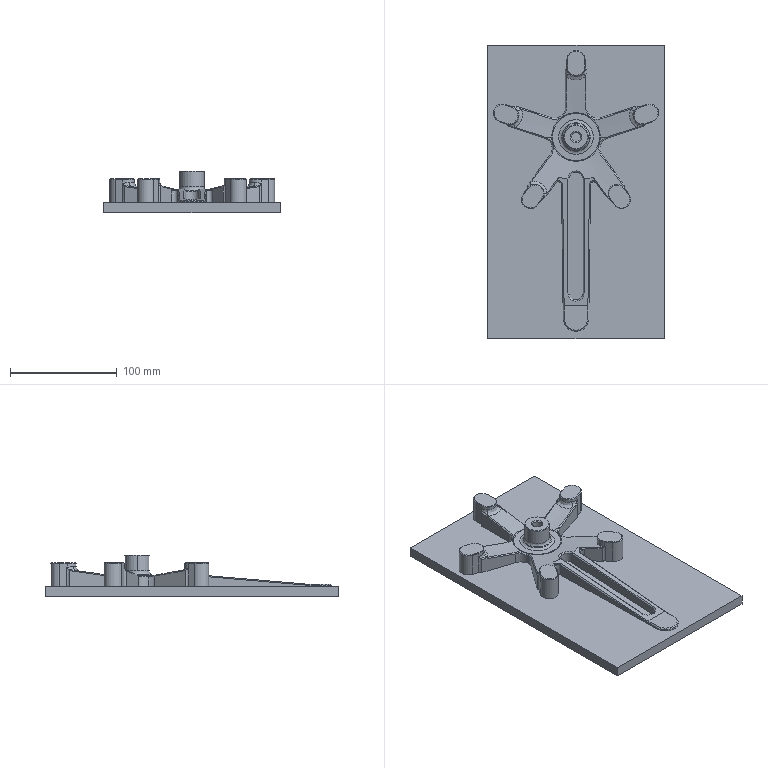NC program | NX | posted with a generic post | part box 165 x 275 x 39 mm
Lines 1 to 1483 of 70117:
N10 G17 G21 G94 G90
(CAVITY_MILL , TOOL : D12)
N12 T00 M6
N14 G54
N16 G17 G0 G90 X0. Y-200.696 S0 M3
N18 G43 Z30. H0
N20 Z2.523
N22 G94 G1 Z-0.477 F250.
N24 Y-189.296
N26 X-82.505
N28 X-82.595 Y-189.281
N30 G2 X-82.781 Y-189.096 R0.471
N32 G1 X-82.796 Y-189.006
N34 Y86.009
N36 G2 X-82.509 Y86.296 R0.293
N38 G1 X82.508
N40 G2 X82.796 Y86.009 R0.293
N42 G1 Y-189.009
N44 G2 X82.508 Y-189.296 R0.293
N46 G1 X0.
N48 Y-183.296
N50 X-76.796
N52 Y80.296
N54 X76.796
N56 Y-183.296
N58 X0.
N60 Y-177.296
N62 X-70.796
N64 Y74.296
N66 X70.796
N68 Y-177.296
N70 X0.
N72 Y-171.296
N74 X-64.796
N76 Y68.296
N78 X64.796
N80 Y-171.296
N82 X0.
N84 Y-165.296
N86 X-58.796
N88 Y62.296
N90 X58.796
N92 Y-165.296
N94 X0.
N96 Y-159.296
N98 X-52.796
N100 Y56.296
N102 X52.796
N104 Y-159.296
N106 X0.
N108 Y-153.296
N110 X-46.796
N112 Y50.296
N114 X46.796
N116 Y-153.296
N118 X0.
N120 Y-147.296
N122 X-40.796
N124 Y44.296
N126 X40.796
N128 Y-147.296
N130 X0.
N132 Y-141.296
N134 X-34.796
N136 Y38.296
N138 X34.796
N140 Y-141.296
N142 X0.
N144 Y-135.296
N146 X-28.796
N148 Y32.296
N150 X28.796
N152 Y-135.296
N154 X0.
N156 Y-129.296
N158 X-22.796
N160 Y26.296
N162 X22.796
N164 Y8.168
N166 X16.796
N168 G3 X-16.796 Y8.168 R18.677
N170 G1 Y20.296
N172 X16.796
N174 Y8.168
N176 X22.796
N178 Y-129.296
N180 X0.
N182 Y-123.296
N184 X-16.796
N186 Y-8.168
N188 G3 X16.796 Y-8.168 R18.677
N190 G1 X15.717 Y-7.643
N192 G2 X-7.643 Y-15.717 R17.477
N194 X15.717 Y-7.643 R-17.477
N196 G1 X16.796 Y-8.168
N198 Y-123.296
N200 X0.
N202 Y-117.296
N204 X-10.796
N206 Y-22.19
N208 G3 X10.796 Y-22.19 R24.677
N210 G1 Y-117.296
N212 X0.
N214 Y-111.296
N216 X-4.796
N218 Y-30.299
N220 G3 X4.796 Y-30.299 R30.677
N222 G1 Y-111.296
N224 X0.
N226 Y-117.296
N228 Z2.523
N230 G0 Z3.
N232 Y-200.696
N234 Z2.047
N236 G1 Z-0.953
N238 Y-189.296
N240 X-82.505
N242 X-82.595 Y-189.281
N244 G2 X-82.781 Y-189.096 R0.471
N246 G1 X-82.796 Y-189.006
N248 Y86.009
N250 G2 X-82.509 Y86.296 R0.293
N252 G1 X82.509
N254 G2 X82.796 Y86.009 R0.293
N256 G1 Y-189.009
N258 G2 X82.508 Y-189.296 R0.293
N260 G1 X0.
N262 Y-183.296
N264 X-76.796
N266 Y80.296
N268 X76.796
N270 Y-183.296
N272 X0.
N274 Y-177.296
N276 X-70.796
N278 Y74.296
N280 X70.796
N282 Y-177.296
N284 X0.
N286 Y-171.296
N288 X-64.796
N290 Y68.296
N292 X64.796
N294 Y-171.296
N296 X0.
N298 Y-165.296
N300 X-58.796
N302 Y62.296
N304 X58.796
N306 Y-165.296
N308 X0.
N310 Y-159.296
N312 X-52.796
N314 Y56.296
N316 X52.796
N318 Y-159.296
N320 X0.
N322 Y-153.296
N324 X-46.796
N326 Y50.296
N328 X46.796
N330 Y-153.296
N332 X0.
N334 Y-147.296
N336 X-40.796
N338 Y44.296
N340 X40.796
N342 Y-147.296
N344 X0.
N346 Y-141.296
N348 X-34.796
N350 Y38.296
N352 X34.796
N354 Y-141.296
N356 X0.
N358 Y-135.296
N360 X-28.796
N362 Y32.296
N364 X28.796
N366 Y-135.296
N368 X0.
N370 Y-129.296
N372 X-22.796
N374 Y26.296
N376 X22.796
N378 Y8.221
N380 X16.796
N382 G3 X-16.796 Y8.221 R18.7
N384 G1 Y20.296
N386 X16.796
N388 Y8.221
N390 X22.796
N392 Y-129.296
N394 X0.
N396 Y-123.296
N398 X-16.796
N400 Y-8.221
N402 G3 X16.796 Y-8.221 R18.7
N404 G1 X15.718 Y-7.694
N406 G2 X-7.694 Y-15.718 R17.5
N408 X15.718 Y-7.694 R-17.5
N410 G1 X16.796 Y-8.221
N412 Y-123.296
N414 X0.
N416 Y-117.296
N418 X-10.796
N420 Y-22.216
N422 G3 X10.796 Y-22.216 R24.7
N424 G1 Y-117.296
N426 X0.
N428 Y-111.296
N430 X-4.796
N432 Y-30.323
N434 G3 X4.796 Y-30.323 R30.7
N436 G1 Y-111.296
N438 X0.
N440 Y-117.296
N442 Z2.047
N444 G0 Z2.523
N446 Y-200.696
N448 Z1.57
N450 G1 Z-1.43
N452 Y-189.296
N454 X-82.505
N456 X-82.595 Y-189.281
N458 G2 X-82.781 Y-189.096 R0.471
N460 G1 X-82.796 Y-189.006
N462 Y86.009
N464 G2 X-82.509 Y86.296 R0.293
N466 G1 X82.509
N468 G2 X82.796 Y86.009 R0.293
N470 G1 Y-189.009
N472 G2 X82.508 Y-189.296 R0.293
N474 G1 X0.
N476 Y-183.296
N478 X-76.796
N480 Y80.296
N482 X76.796
N484 Y-183.296
N486 X0.
N488 Y-177.296
N490 X-70.796
N492 Y74.296
N494 X70.796
N496 Y-177.296
N498 X0.
N500 Y-171.296
N502 X-64.796
N504 Y68.296
N506 X64.796
N508 Y-171.296
N510 X0.
N512 Y-165.296
N514 X-58.796
N516 Y62.296
N518 X58.796
N520 Y-165.296
N522 X0.
N524 Y-159.296
N526 X-52.796
N528 Y56.296
N530 X52.796
N532 Y-159.296
N534 X0.
N536 Y-153.296
N538 X-46.796
N540 Y50.296
N542 X46.796
N544 Y-153.296
N546 X0.
N548 Y-147.296
N550 X-40.796
N552 Y44.296
N554 X40.796
N556 Y-147.296
N558 X0.
N560 Y-141.296
N562 X-34.796
N564 Y38.296
N566 X34.796
N568 Y-141.296
N570 X0.
N572 Y-135.296
N574 X-28.796
N576 Y32.296
N578 X28.796
N580 Y-135.296
N582 X0.
N584 Y-129.296
N586 X-22.796
N588 Y26.296
N590 X22.796
N592 Y8.221
N594 X16.796
N596 G3 X-16.796 Y8.221 R18.7
N598 G1 Y20.296
N600 X16.796
N602 Y8.221
N604 X22.796
N606 Y-129.296
N608 X0.
N610 Y-123.296
N612 X-16.796
N614 Y-8.221
N616 G3 X16.796 Y-8.221 R18.7
N618 G1 X15.718 Y-7.694
N620 G2 X-7.694 Y-15.718 R17.5
N622 X15.718 Y-7.694 R-17.5
N624 G1 X16.796 Y-8.221
N626 Y-123.296
N628 X0.
N630 Y-117.296
N632 X-10.796
N634 Y-22.216
N636 G3 X10.796 Y-22.216 R24.7
N638 G1 Y-117.296
N640 X0.
N642 Y-111.296
N644 X-4.796
N646 Y-30.323
N648 G3 X4.796 Y-30.323 R30.7
N650 G1 Y-111.296
N652 X0.
N654 Y-117.296
N656 Z1.57
N658 G0 Z2.047
N660 Y-200.696
N662 Z1.093
N664 G1 Z-1.907
N666 Y-189.296
N668 X-82.505
N670 X-82.595 Y-189.281
N672 G2 X-82.78 Y-189.096 R0.471
N674 G1 X-82.796 Y-189.006
N676 Y86.009
N678 G2 X-82.509 Y86.296 R0.293
N680 G1 X82.509
N682 G2 X82.796 Y86.009 R0.293
N684 G1 Y-189.009
N686 G2 X82.508 Y-189.296 R0.293
N688 G1 X0.
N690 Y-183.296
N692 X-76.796
N694 Y80.296
N696 X76.796
N698 Y-183.296
N700 X0.
N702 Y-177.296
N704 X-70.796
N706 Y74.296
N708 X70.796
N710 Y-177.296
N712 X0.
N714 Y-171.296
N716 X-64.796
N718 Y68.296
N720 X64.796
N722 Y-171.296
N724 X0.
N726 Y-165.296
N728 X-58.796
N730 Y62.296
N732 X58.796
N734 Y-165.296
N736 X0.
N738 Y-159.296
N740 X-52.796
N742 Y56.296
N744 X52.796
N746 Y-159.296
N748 X0.
N750 Y-153.296
N752 X-46.796
N754 Y50.296
N756 X46.796
N758 Y-153.296
N760 X0.
N762 Y-147.296
N764 X-40.796
N766 Y44.296
N768 X40.796
N770 Y-147.296
N772 X0.
N774 Y-141.296
N776 X-34.796
N778 Y38.296
N780 X34.796
N782 Y-141.296
N784 X0.
N786 Y-135.296
N788 X-28.796
N790 Y32.296
N792 X28.796
N794 Y-135.296
N796 X0.
N798 Y-129.296
N800 X-22.796
N802 Y26.296
N804 X22.796
N806 Y8.221
N808 X16.796
N810 G3 X-16.796 Y8.221 R18.7
N812 G1 Y20.296
N814 X16.796
N816 Y8.221
N818 X22.796
N820 Y-129.296
N822 X0.
N824 Y-123.296
N826 X-16.796
N828 Y-8.221
N830 G3 X16.796 Y-8.221 R18.7
N832 G1 X15.718 Y-7.694
N834 G2 X-7.694 Y-15.718 R17.5
N836 X15.718 Y-7.694 R-17.5
N838 G1 X16.796 Y-8.221
N840 Y-123.296
N842 X0.
N844 Y-117.296
N846 X-10.796
N848 Y-22.216
N850 G3 X10.796 Y-22.216 R24.7
N852 G1 Y-117.296
N854 X0.
N856 Y-111.296
N858 X-4.796
N860 Y-30.323
N862 G3 X4.796 Y-30.323 R30.7
N864 G1 Y-111.296
N866 X0.
N868 Y-117.296
N870 Z1.093
N872 G0 Z1.57
N874 Y-200.696
N876 Z0.617
N878 G1 Z-2.383
N880 Y-189.296
N882 X-82.505
N884 X-82.595 Y-189.281
N886 G2 X-82.78 Y-189.096 R0.471
N888 G1 X-82.796 Y-189.006
N890 Y86.009
N892 G2 X-82.509 Y86.296 R0.293
N894 G1 X82.509
N896 G2 X82.796 Y86.009 R0.293
N898 G1 Y-189.009
N900 G2 X82.508 Y-189.296 R0.293
N902 G1 X0.
N904 Y-183.296
N906 X-76.796
N908 Y80.296
N910 X76.796
N912 Y-183.296
N914 X0.
N916 Y-177.296
N918 X-70.796
N920 Y74.296
N922 X70.796
N924 Y-177.296
N926 X0.
N928 Y-171.296
N930 X-64.796
N932 Y68.296
N934 X64.796
N936 Y-171.296
N938 X0.
N940 Y-165.296
N942 X-58.796
N944 Y62.296
N946 X58.796
N948 Y-165.296
N950 X0.
N952 Y-159.296
N954 X-52.796
N956 Y56.296
N958 X52.796
N960 Y-159.296
N962 X0.
N964 Y-153.296
N966 X-46.796
N968 Y50.296
N970 X46.796
N972 Y-153.296
N974 X0.
N976 Y-147.296
N978 X-40.796
N980 Y44.296
N982 X40.796
N984 Y-147.296
N986 X0.
N988 Y-141.296
N990 X-34.796
N992 Y38.296
N994 X34.796
N996 Y-141.296
N998 X0.
N1000 Y-135.296
N1002 X-28.796
N1004 Y32.296
N1006 X28.796
N1008 Y-135.296
N1010 X0.
N1012 Y-129.296
N1014 X-22.796
N1016 Y26.296
N1018 X22.796
N1020 Y8.221
N1022 X16.796
N1024 G3 X-16.796 Y8.221 R18.7
N1026 G1 Y20.296
N1028 X16.796
N1030 Y8.221
N1032 X22.796
N1034 Y-129.296
N1036 X0.
N1038 Y-123.296
N1040 X-16.796
N1042 Y-8.221
N1044 G3 X16.796 Y-8.221 R18.7
N1046 G1 X15.718 Y-7.693
N1048 G2 X-7.693 Y-15.718 R17.5
N1050 X15.718 Y-7.693 R-17.5
N1052 G1 X16.796 Y-8.221
N1054 Y-123.296
N1056 X0.
N1058 Y-117.296
N1060 X-10.796
N1062 Y-22.216
N1064 G3 X10.796 Y-22.216 R24.7
N1066 G1 Y-117.296
N1068 X0.
N1070 Y-111.296
N1072 X-4.796
N1074 Y-30.323
N1076 G3 X4.796 Y-30.323 R30.7
N1078 G1 Y-111.296
N1080 X0.
N1082 Y-117.296
N1084 Z0.617
N1086 G0 Z1.093
N1088 Y-200.696
N1090 Z0.14
N1092 G1 Z-2.86
N1094 Y-189.296
N1096 X-82.505
N1098 X-82.595 Y-189.281
N1100 G2 X-82.78 Y-189.096 R0.471
N1102 G1 X-82.796 Y-189.006
N1104 Y86.009
N1106 G2 X-82.509 Y86.296 R0.293
N1108 G1 X82.509
N1110 G2 X82.796 Y86.009 R0.293
N1112 G1 Y-189.009
N1114 G2 X82.508 Y-189.296 R0.293
N1116 G1 X0.
N1118 Y-183.296
N1120 X-76.796
N1122 Y80.296
N1124 X76.796
N1126 Y-183.296
N1128 X0.
N1130 Y-177.296
N1132 X-70.796
N1134 Y74.296
N1136 X70.796
N1138 Y-177.296
N1140 X0.
N1142 Y-171.296
N1144 X-64.796
N1146 Y68.296
N1148 X64.796
N1150 Y-171.296
N1152 X0.
N1154 Y-165.296
N1156 X-58.796
N1158 Y62.296
N1160 X58.796
N1162 Y-165.296
N1164 X0.
N1166 Y-159.296
N1168 X-52.796
N1170 Y56.296
N1172 X52.796
N1174 Y-159.296
N1176 X0.
N1178 Y-153.296
N1180 X-46.796
N1182 Y50.296
N1184 X46.796
N1186 Y-153.296
N1188 X0.
N1190 Y-147.296
N1192 X-40.796
N1194 Y44.296
N1196 X40.796
N1198 Y-147.296
N1200 X0.
N1202 Y-141.296
N1204 X-34.796
N1206 Y38.296
N1208 X34.796
N1210 Y-141.296
N1212 X0.
N1214 Y-135.296
N1216 X-28.796
N1218 Y32.296
N1220 X28.796
N1222 Y-135.296
N1224 X0.
N1226 Y-129.296
N1228 X-22.796
N1230 Y26.296
N1232 X22.796
N1234 Y8.221
N1236 X16.796
N1238 G3 X-16.796 Y8.221 R18.7
N1240 G1 Y20.296
N1242 X16.796
N1244 Y8.221
N1246 X22.796
N1248 Y-129.296
N1250 X0.
N1252 Y-123.296
N1254 X-16.796
N1256 Y-8.221
N1258 G3 X16.796 Y-8.221 R18.7
N1260 G1 X15.718 Y-7.693
N1262 G2 X-7.693 Y-15.718 R17.5
N1264 X15.718 Y-7.693 R-17.5
N1266 G1 X16.796 Y-8.221
N1268 Y-123.296
N1270 X0.
N1272 Y-117.296
N1274 X-10.796
N1276 Y-22.216
N1278 G3 X10.796 Y-22.216 R24.7
N1280 G1 Y-117.296
N1282 X0.
N1284 Y-111.296
N1286 X-4.796
N1288 Y-30.323
N1290 G3 X4.796 Y-30.323 R30.7
N1292 G1 Y-111.296
N1294 X0.
N1296 Y-117.296
N1298 Z0.14
N1300 G0 Z0.617
N1302 Y-200.696
N1304 Z-0.337
N1306 G1 Z-3.337
N1308 Y-189.296
N1310 X-82.505
N1312 X-82.595 Y-189.281
N1314 G2 X-82.78 Y-189.096 R0.471
N1316 G1 X-82.796 Y-189.006
N1318 Y86.009
N1320 G2 X-82.509 Y86.296 R0.293
N1322 G1 X82.509
N1324 G2 X82.796 Y86.009 R0.293
N1326 G1 Y-189.009
N1328 G2 X82.508 Y-189.296 R0.293
N1330 G1 X0.
N1332 Y-183.296
N1334 X-76.796
N1336 Y80.296
N1338 X76.796
N1340 Y-183.296
N1342 X0.
N1344 Y-177.296
N1346 X-70.796
N1348 Y74.296
N1350 X70.796
N1352 Y-177.296
N1354 X0.
N1356 Y-171.296
N1358 X-64.796
N1360 Y68.296
N1362 X64.796
N1364 Y-171.296
N1366 X0.
N1368 Y-165.296
N1370 X-58.796
N1372 Y62.296
N1374 X58.796
N1376 Y-165.296
N1378 X0.
N1380 Y-159.296
N1382 X-52.796
N1384 Y56.296
N1386 X52.796
N1388 Y-159.296
N1390 X0.
N1392 Y-153.296
N1394 X-46.796
N1396 Y50.296
N1398 X46.796
N1400 Y-153.296
N1402 X0.
N1404 Y-147.296
N1406 X-40.796
N1408 Y44.296
N1410 X40.796
N1412 Y-147.296
N1414 X0.
N1416 Y-141.296
N1418 X-34.796
N1420 Y38.296
N1422 X34.796
N1424 Y-141.296
N1426 X0.
N1428 Y-135.296
N1430 X-28.796
N1432 Y32.296
N1434 X28.796
N1436 Y-135.296
N1438 X0.
N1440 Y-129.296
N1442 X-22.796
N1444 Y26.296
N1446 X22.796
N1448 Y8.221
N1450 X16.796
N1452 G3 X-16.796 Y8.221 R18.7
N1454 G1 Y20.296
N1456 X16.796
N1458 Y8.221
N1460 X22.796
N1462 Y-129.296
N1464 X0.
N1466 Y-123.296
N1468 X-16.796
N1470 Y-8.221
N1472 G3 X16.796 Y-8.221 R18.7
N1474 G1 X15.718 Y-7.693
N1476 G2 X-7.693 Y-15.718 R17.5
N1478 X15.718 Y-7.693 R-17.5
N1480 G1 X16.796 Y-8.221
N1482 Y-123.296
N1484 X0.
N1486 Y-117.296
N1488 X-10.796
N1490 Y-22.216
N1492 G3 X10.796 Y-22.216 R24.7
N1494 G1 Y-117.296
N1496 X0.
N1498 Y-111.296
N1500 X-4.796
N1502 Y-30.323
N1504 G3 X4.796 Y-30.323 R30.7
N1506 G1 Y-111.296
N1508 X0.
N1510 Y-117.296
N1512 Z-0.337
N1514 G0 Z0.14
N1516 Y-200.697
N1518 Z-0.813
N1520 G1 Z-3.813
N1522 Y-189.297
N1524 X-82.505
N1526 X-82.595 Y-189.281
N1528 G2 X-82.78 Y-189.096 R0.471
N1530 G1 X-82.796 Y-189.006
N1532 Y86.009
N1534 G2 X-82.509 Y86.296 R0.293
N1536 G1 X82.509
N1538 G2 X82.796 Y86.009 R0.293
N1540 G1 Y-189.009
N1542 G2 X82.508 Y-189.297 R0.293
N1544 G1 X0.
N1546 Y-183.297
N1548 X-76.796
N1550 Y80.296
N1552 X76.796
N1554 Y-183.297
N1556 X0.
N1558 Y-177.297
N1560 X-70.796
N1562 Y74.296
N1564 X70.796
N1566 Y-177.297
N1568 X0.
N1570 Y-171.297
N1572 X-64.796
N1574 Y68.296
N1576 X64.796
N1578 Y-171.297
N1580 X0.
N1582 Y-165.297
N1584 X-58.796
N1586 Y62.296
N1588 X58.796
N1590 Y-165.297
N1592 X0.
N1594 Y-159.297
N1596 X-52.796
N1598 Y56.296
N1600 X52.796
N1602 Y-159.297
N1604 X0.
N1606 Y-153.297
N1608 X-46.796
N1610 Y50.296
N1612 X46.796
N1614 Y-153.297
N1616 X0.
N1618 Y-147.297
N1620 X-40.796
N1622 Y44.296
N1624 X40.796
N1626 Y-147.297
N1628 X0.
N1630 Y-141.297
N1632 X-34.796
N1634 Y38.296
N1636 X34.796
N1638 Y-141.297
N1640 X0.
N1642 Y-135.297
N1644 X-28.796
N1646 Y32.296
N1648 X28.796
N1650 Y-135.297
N1652 X0.
N1654 Y-129.297
N1656 X-22.796
N1658 Y26.296
N1660 X22.796
N1662 Y8.221
N1664 X16.796
N1666 G3 X-16.796 Y8.221 R18.7
N1668 G1 Y20.296
N1670 X16.796
N1672 Y8.221
N1674 X22.796
N1676 Y-129.297
N1678 X0.
N1680 Y-123.297
N1682 X-16.796
N1684 Y-8.221
N1686 G3 X16.796 Y-8.221 R18.7
N1688 G1 X15.718 Y-7.693
N1690 G2 X-7.693 Y-15.718 R17.5
N1692 X15.718 Y-7.693 R-17.5
N1694 G1 X16.796 Y-8.221
N1696 Y-123.297
N1698 X0.
N1700 Y-117.297
N1702 X-10.796
N1704 Y-22.216
N1706 G3 X10.796 Y-22.216 R24.7
N1708 G1 Y-117.297
N1710 X0.
N1712 Y-111.297
N1714 X-4.796
N1716 Y-30.323
N1718 G3 X4.796 Y-30.323 R30.7
N1720 G1 Y-111.297
N1722 X0.
N1724 Y-117.297
N1726 Z-0.813
N1728 G0 Z-0.337
N1730 Y-200.697
N1732 Z-1.29
N1734 G1 Z-4.29
N1736 Y-189.297
N1738 X-82.505
N1740 X-82.595 Y-189.281
N1742 G2 X-82.781 Y-189.096 R0.471
N1744 G1 X-82.796 Y-189.006
N1746 Y86.009
N1748 G2 X-82.509 Y86.296 R0.293
N1750 G1 X82.509
N1752 G2 X82.796 Y86.009 R0.293
N1754 G1 Y-189.009
N1756 G2 X82.508 Y-189.297 R0.293
N1758 G1 X0.
N1760 Y-183.297
N1762 X-76.796
N1764 Y80.296
N1766 X76.796
N1768 Y-183.297
N1770 X0.
N1772 Y-177.297
N1774 X-70.796
N1776 Y74.296
N1778 X70.796
N1780 Y-177.297
N1782 X0.
N1784 Y-171.297
N1786 X-64.796
N1788 Y68.296
N1790 X64.796
N1792 Y-171.297
N1794 X0.
N1796 Y-165.297
N1798 X-58.796
N1800 Y62.296
N1802 X58.796
N1804 Y-165.297
N1806 X0.
N1808 Y-159.297
N1810 X-52.796
N1812 Y56.296
N1814 X52.796
N1816 Y-159.297
N1818 X0.
N1820 Y-153.297
N1822 X-46.796
N1824 Y50.296
N1826 X46.796
N1828 Y-153.297
N1830 X0.
N1832 Y-147.297
N1834 X-40.796
N1836 Y44.296
N1838 X40.796
N1840 Y-147.297
N1842 X0.
N1844 Y-141.297
N1846 X-34.796
N1848 Y38.296
N1850 X34.796
N1852 Y-141.297
N1854 X0.
N1856 Y-135.297
N1858 X-28.796
N1860 Y32.296
N1862 X28.796
N1864 Y-135.297
N1866 X0.
N1868 Y-129.297
N1870 X-22.796
N1872 Y26.296
N1874 X22.796
N1876 Y8.221
N1878 X16.796
N1880 G3 X-16.796 Y8.221 R18.7
N1882 G1 Y20.296
N1884 X16.796
N1886 Y8.221
N1888 X22.796
N1890 Y-129.297
N1892 X0.
N1894 Y-123.297
N1896 X-16.796
N1898 Y-8.221
N1900 G3 X16.796 Y-8.221 R18.7
N1902 G1 X15.718 Y-7.693
N1904 G2 X-7.693 Y-15.718 R17.5
N1906 X15.718 Y-7.693 R-17.5
N1908 G1 X16.796 Y-8.221
N1910 Y-123.297
N1912 X0.
N1914 Y-117.297
N1916 X-10.796
N1918 Y-22.216
N1920 G3 X10.796 Y-22.216 R24.7
N1922 G1 Y-117.297
N1924 X0.
N1926 Y-111.297
N1928 X-4.796
N1930 Y-30.323
N1932 G3 X4.796 Y-30.323 R30.7
N1934 G1 Y-111.297
N1936 X0.
N1938 Y-117.297
N1940 Z-1.29
N1942 G0 Z-0.813
N1944 Y-200.697
N1946 Z-1.767
N1948 G1 Z-4.767
N1950 Y-189.297
N1952 X-82.505
N1954 X-82.595 Y-189.281
N1956 G2 X-82.781 Y-189.096 R0.471
N1958 G1 X-82.796 Y-189.006
N1960 Y86.009
N1962 G2 X-82.509 Y86.296 R0.293
N1964 G1 X82.509
N1966 G2 X82.796 Y86.009 R0.293
N1968 G1 Y-189.009
N1970 G2 X82.508 Y-189.297 R0.293
N1972 G1 X0.
N1974 Y-183.297
N1976 X-76.796
N1978 Y80.296
N1980 X76.796
N1982 Y-183.297
N1984 X0.
N1986 Y-177.297
N1988 X-70.796
N1990 Y74.296
N1992 X70.796
N1994 Y-177.297
N1996 X0.
N1998 Y-171.297
N2000 X-64.796
N2002 Y68.296
N2004 X64.796
N2006 Y-171.297
N2008 X0.
N2010 Y-165.297
N2012 X-58.796
N2014 Y62.296
N2016 X58.796
N2018 Y-165.297
N2020 X0.
N2022 Y-159.297
N2024 X-52.796
N2026 Y56.296
N2028 X52.796
N2030 Y-159.297
N2032 X0.
N2034 Y-153.297
N2036 X-46.796
N2038 Y50.296
N2040 X46.796
N2042 Y-153.297
N2044 X0.
N2046 Y-147.297
N2048 X-40.796
N2050 Y44.296
N2052 X40.796
N2054 Y-147.297
N2056 X0.
N2058 Y-141.297
N2060 X-34.796
N2062 Y38.296
N2064 X34.796
N2066 Y-141.297
N2068 X0.
N2070 Y-135.297
N2072 X-28.796
N2074 Y32.296
N2076 X28.796
N2078 Y-135.297
N2080 X0.
N2082 Y-129.297
N2084 X-22.796
N2086 Y26.296
N2088 X22.796
N2090 Y8.221
N2092 X16.796
N2094 G3 X-16.796 Y8.221 R18.7
N2096 G1 Y20.296
N2098 X16.796
N2100 Y8.221
N2102 X22.796
N2104 Y-129.297
N2106 X0.
N2108 Y-123.297
N2110 X-16.796
N2112 Y-8.221
N2114 G3 X16.796 Y-8.221 R18.7
N2116 G1 X15.718 Y-7.693
N2118 G2 X-7.693 Y-15.718 R17.5
N2120 X15.718 Y-7.693 R-17.5
N2122 G1 X16.796 Y-8.221
N2124 Y-123.297
N2126 X0.
N2128 Y-117.297
N2130 X-10.796
N2132 Y-22.216
N2134 G3 X10.796 Y-22.216 R24.7
N2136 G1 Y-117.297
N2138 X0.
N2140 Y-111.297
N2142 X-4.796
N2144 Y-30.323
N2146 G3 X4.796 Y-30.323 R30.7
N2148 G1 Y-111.297
N2150 X0.
N2152 Y-117.297
N2154 Z-1.767
N2156 G0 Z-1.29
N2158 Y-200.697
N2160 Z-2.243
N2162 G1 Z-5.243
N2164 Y-189.297
N2166 X-82.505
N2168 X-82.595 Y-189.281
N2170 G2 X-82.781 Y-189.096 R0.472
N2172 G1 X-82.796 Y-189.006
N2174 Y86.009
N2176 G2 X-82.509 Y86.296 R0.293
N2178 G1 X82.509
N2180 G2 X82.796 Y86.009 R0.293
N2182 G1 Y-189.009
N2184 G2 X82.508 Y-189.297 R0.293
N2186 G1 X0.
N2188 Y-183.297
N2190 X-76.796
N2192 Y80.296
N2194 X76.796
N2196 Y-183.297
N2198 X0.
N2200 Y-177.297
N2202 X-70.796
N2204 Y74.296
N2206 X70.796
N2208 Y-177.297
N2210 X0.
N2212 Y-171.297
N2214 X-64.796
N2216 Y68.296
N2218 X64.796
N2220 Y-171.297
N2222 X0.
N2224 Y-165.297
N2226 X-58.796
N2228 Y62.296
N2230 X58.796
N2232 Y-165.297
N2234 X0.
N2236 Y-159.297
N2238 X-52.796
N2240 Y56.296
N2242 X52.796
N2244 Y-159.297
N2246 X0.
N2248 Y-153.297
N2250 X-46.796
N2252 Y50.296
N2254 X46.796
N2256 Y-153.297
N2258 X0.
N2260 Y-147.297
N2262 X-40.796
N2264 Y44.296
N2266 X40.796
N2268 Y-147.297
N2270 X0.
N2272 Y-141.297
N2274 X-34.796
N2276 Y38.296
N2278 X34.796
N2280 Y-141.297
N2282 X0.
N2284 Y-135.297
N2286 X-28.796
N2288 Y32.296
N2290 X28.796
N2292 Y-135.297
N2294 X0.
N2296 Y-129.297
N2298 X-22.796
N2300 Y26.296
N2302 X22.796
N2304 Y8.22
N2306 X16.796
N2308 G3 X-16.796 Y8.22 R18.7
N2310 G1 Y20.296
N2312 X16.796
N2314 Y8.22
N2316 X22.796
N2318 Y-129.297
N2320 X0.
N2322 Y-123.297
N2324 X-16.796
N2326 Y-8.221
N2328 G3 X16.796 Y-8.221 R18.7
N2330 G1 X15.718 Y-7.693
N2332 G2 X-7.693 Y-15.718 R17.5
N2334 X15.718 Y-7.693 R-17.5
N2336 G1 X16.796 Y-8.221
N2338 Y-123.297
N2340 X0.
N2342 Y-117.297
N2344 X-10.796
N2346 Y-22.216
N2348 G3 X10.796 Y-22.216 R24.7
N2350 G1 Y-117.297
N2352 X0.
N2354 Y-111.297
N2356 X-4.796
N2358 Y-30.323
N2360 G3 X4.796 Y-30.323 R30.7
N2362 G1 Y-111.297
N2364 X0.
N2366 Y-117.297
N2368 Z-2.243
N2370 G0 Z-1.767
N2372 Y-200.697
N2374 Z-2.72
N2376 G1 Z-5.72
N2378 Y-189.297
N2380 X-82.505
N2382 X-82.595 Y-189.281
N2384 G2 X-82.781 Y-189.096 R0.472
N2386 G1 X-82.796 Y-189.006
N2388 Y86.009
N2390 G2 X-82.509 Y86.296 R0.293
N2392 G1 X82.509
N2394 G2 X82.796 Y86.009 R0.293
N2396 G1 Y-189.009
N2398 G2 X82.508 Y-189.297 R0.293
N2400 G1 X0.
N2402 Y-183.297
N2404 X-76.796
N2406 Y80.296
N2408 X76.796
N2410 Y-183.297
N2412 X0.
N2414 Y-177.297
N2416 X-70.796
N2418 Y74.296
N2420 X70.796
N2422 Y-177.297
N2424 X0.
N2426 Y-171.297
N2428 X-64.796
N2430 Y68.296
N2432 X64.796
N2434 Y-171.297
N2436 X0.
N2438 Y-165.297
N2440 X-58.796
N2442 Y62.296
N2444 X58.796
N2446 Y-165.297
N2448 X0.
N2450 Y-159.297
N2452 X-52.796
N2454 Y56.296
N2456 X52.796
N2458 Y-159.297
N2460 X0.
N2462 Y-153.297
N2464 X-46.796
N2466 Y50.296
N2468 X46.796
N2470 Y-153.297
N2472 X0.
N2474 Y-147.297
N2476 X-40.796
N2478 Y44.296
N2480 X40.796
N2482 Y-147.297
N2484 X0.
N2486 Y-141.297
N2488 X-34.796
N2490 Y38.296
N2492 X34.796
N2494 Y-141.297
N2496 X0.
N2498 Y-135.297
N2500 X-28.796
N2502 Y32.296
N2504 X28.796
N2506 Y-135.297
N2508 X0.
N2510 Y-129.297
N2512 X-22.796
N2514 Y26.296
N2516 X22.796
N2518 Y8.22
N2520 X16.796
N2522 G3 X-16.796 Y8.22 R18.7
N2524 G1 Y20.296
N2526 X16.796
N2528 Y8.22
N2530 X22.796
N2532 Y-129.297
N2534 X0.
N2536 Y-123.297
N2538 X-16.796
N2540 Y-8.22
N2542 G3 X16.796 Y-8.22 R18.7
N2544 G1 X15.718 Y-7.693
N2546 G2 X-7.693 Y-15.718 R17.5
N2548 X15.718 Y-7.693 R-17.5
N2550 G1 X16.796 Y-8.22
N2552 Y-123.297
N2554 X0.
N2556 Y-117.297
N2558 X-10.796
N2560 Y-22.216
N2562 G3 X10.796 Y-22.216 R24.7
N2564 G1 Y-117.297
N2566 X0.
N2568 Y-111.297
N2570 X-4.796
N2572 Y-30.323
N2574 G3 X4.796 Y-30.323 R30.7
N2576 G1 Y-111.297
N2578 X0.
N2580 Y-117.297
N2582 Z-2.72
N2584 G0 Z-2.243
N2586 Y-200.697
N2588 Z-3.197
N2590 G1 Z-6.197
N2592 Y-189.297
N2594 X-82.505
N2596 X-82.595 Y-189.281
N2598 G2 X-82.781 Y-189.096 R0.472
N2600 G1 X-82.796 Y-189.006
N2602 Y86.009
N2604 G2 X-82.509 Y86.296 R0.293
N2606 G1 X82.509
N2608 G2 X82.796 Y86.009 R0.293
N2610 G1 Y-189.009
N2612 G2 X82.508 Y-189.297 R0.293
N2614 G1 X0.
N2616 Y-183.297
N2618 X-76.796
N2620 Y80.296
N2622 X76.796
N2624 Y-183.297
N2626 X0.
N2628 Y-177.297
N2630 X-70.796
N2632 Y74.296
N2634 X70.796
N2636 Y-177.297
N2638 X0.
N2640 Y-171.297
N2642 X-64.796
N2644 Y68.296
N2646 X64.796
N2648 Y-171.297
N2650 X0.
N2652 Y-165.297
N2654 X-58.796
N2656 Y62.296
N2658 X58.796
N2660 Y-165.297
N2662 X0.
N2664 Y-159.297
N2666 X-52.796
N2668 Y56.296
N2670 X52.796
N2672 Y-159.297
N2674 X0.
N2676 Y-153.297
N2678 X-46.796
N2680 Y50.296
N2682 X46.796
N2684 Y-153.297
N2686 X0.
N2688 Y-147.297
N2690 X-40.796
N2692 Y44.296
N2694 X40.796
N2696 Y-147.297
N2698 X0.
N2700 Y-141.297
N2702 X-34.796
N2704 Y38.296
N2706 X34.796
N2708 Y-141.297
N2710 X0.
N2712 Y-135.297
N2714 X-28.796
N2716 Y32.296
N2718 X28.796
N2720 Y-135.297
N2722 X0.
N2724 Y-129.297
N2726 X-22.796
N2728 Y26.296
N2730 X22.796
N2732 Y8.22
N2734 X16.796
N2736 G3 X-16.796 Y8.22 R18.7
N2738 G1 Y20.296
N2740 X16.796
N2742 Y8.22
N2744 X22.796
N2746 Y-129.297
N2748 X0.
N2750 Y-123.297
N2752 X-16.796
N2754 Y-8.22
N2756 G3 X16.796 Y-8.22 R18.7
N2758 G1 X15.718 Y-7.693
N2760 G2 X-7.693 Y-15.718 R17.5
N2762 X15.718 Y-7.693 R-17.5
N2764 G1 X16.796 Y-8.22
N2766 Y-123.297
N2768 X0.
N2770 Y-117.297
N2772 X-10.796
N2774 Y-22.216
N2776 G3 X10.796 Y-22.216 R24.7
N2778 G1 Y-117.297
N2780 X0.
N2782 Y-111.297
N2784 X-4.796
N2786 Y-30.323
N2788 G3 X4.796 Y-30.323 R30.7
N2790 G1 Y-111.297
N2792 X0.
N2794 Y-117.297
N2796 Z-3.197
N2798 G0 Z-2.72
N2800 Y-200.697
N2802 Z-3.673
N2804 G1 Z-6.673
N2806 Y-189.297
N2808 X-82.505
N2810 X-82.595 Y-189.281
N2812 G2 X-82.781 Y-189.096 R0.473
N2814 G1 X-82.796 Y-189.006
N2816 X-82.797 Y86.009
N2818 G2 X-82.509 Y86.296 R0.293
N2820 G1 X82.509
N2822 G2 X82.797 Y86.009 R0.293
N2824 G1 X82.796 Y-189.009
N2826 G2 X82.508 Y-189.297 R0.293
N2828 G1 X0.
N2830 Y-183.297
N2832 X-76.796
N2834 X-76.797 Y80.296
N2836 X76.797
N2838 X76.796 Y-183.297
N2840 X0.
N2842 Y-177.297
N2844 X-70.796
N2846 X-70.797 Y74.296
N2848 X70.797
N2850 X70.796 Y-177.297
N2852 X0.
N2854 Y-171.297
N2856 X-64.796
N2858 X-64.797 Y68.296
N2860 X64.797
N2862 X64.796 Y-171.297
N2864 X0.
N2866 Y-165.297
N2868 X-58.796
N2870 Y62.296
N2872 X58.796
N2874 Y-165.297
N2876 X0.
N2878 Y-159.297
N2880 X-52.796
N2882 Y56.296
N2884 X52.796
N2886 Y-159.297
N2888 X0.
N2890 Y-153.297
N2892 X-46.796
N2894 Y50.296
N2896 X46.796
N2898 Y-153.297
N2900 X0.
N2902 Y-147.297
N2904 X-40.796
N2906 Y44.296
N2908 X40.796
N2910 Y-147.297
N2912 X0.
N2914 Y-141.297
N2916 X-34.796
N2918 Y38.296
N2920 X34.796
N2922 Y-141.297
N2924 X0.
N2926 Y-135.297
N2928 X-28.796
N2930 Y32.296
N2932 X28.796
N2934 Y-135.297
N2936 X0.
N2938 Y-129.297
N2940 X-22.796
N2942 Y26.296
N2944 X22.796
N2946 Y8.22
N2948 X16.796
N2950 G3 X-16.796 Y8.22 R18.7
N2952 G1 Y20.296
N2954 X16.796
N2956 Y8.22
N2958 X22.796
N2960 Y-129.297
N2962 X0.
N2964 Y-123.297